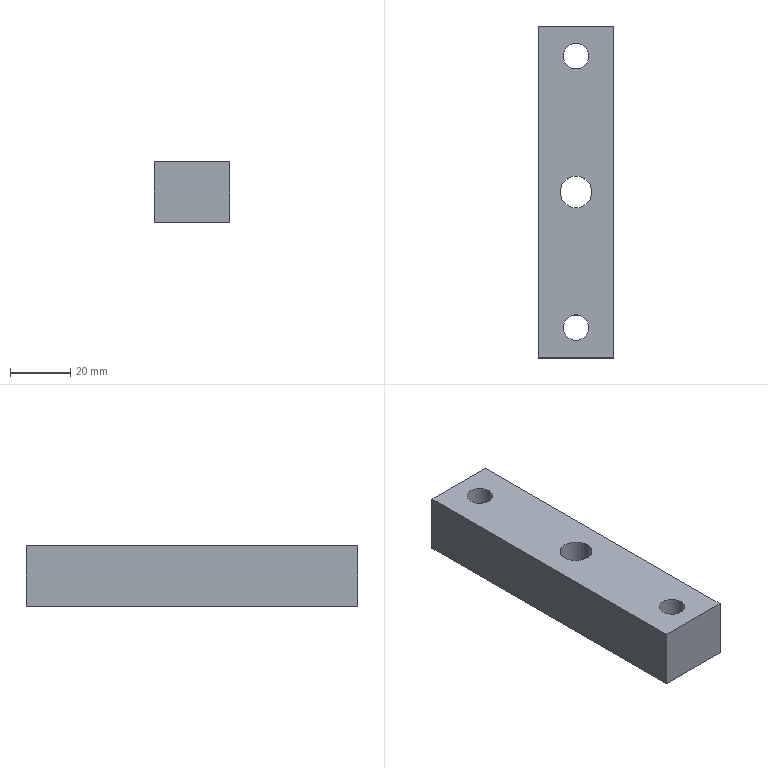Part | SolidWorks | features ICE 2, Extrusion 1, HoleWzd 1 | 1 solid | 18 faces | box 25 x 110 x 20 mm | volume 49479 mm3 | cylinder 10 | plane 8 | commonest cylinder face diameters 8.5 x4 13 x4 10.5 x2
STEP:
#1=CARTESIAN_POINT('',(5.25,0.,20.));
#2=VERTEX_POINT('',#1);
#3=CARTESIAN_POINT('',(-5.25,0.,20.));
#4=VERTEX_POINT('',#3);
#5=CARTESIAN_POINT('',(0.,0.,20.));
#6=DIRECTION('',(0.,0.,-1.));
#7=DIRECTION('',(-1.,0.,0.));
#8=AXIS2_PLACEMENT_3D('',#5,#6,#7);
#9=CIRCLE('',#8,5.25);
#10=EDGE_CURVE('',#2,#4,#9,.T.);
#11=ORIENTED_EDGE('',*,*,#10,.F.);
#12=CARTESIAN_POINT('',(5.25,0.,0.));
#13=VERTEX_POINT('',#12);
#14=CARTESIAN_POINT('',(5.25,0.,0.));
#15=DIRECTION('',(0.,0.,-1.));
#16=VECTOR('',#15,1000.);
#17=LINE('',#14,#16);
#18=EDGE_CURVE('',#2,#13,#17,.T.);
#19=ORIENTED_EDGE('',*,*,#18,.T.);
#20=CARTESIAN_POINT('',(-5.25,0.,0.));
#21=VERTEX_POINT('',#20);
#22=CARTESIAN_POINT('',(0.,0.,0.));
#23=DIRECTION('',(0.,0.,-1.));
#24=DIRECTION('',(-1.,0.,0.));
#25=AXIS2_PLACEMENT_3D('',#22,#23,#24);
#26=CIRCLE('',#25,5.25);
#27=EDGE_CURVE('',#13,#21,#26,.T.);
#28=ORIENTED_EDGE('',*,*,#27,.T.);
#29=CARTESIAN_POINT('',(-5.25,0.,0.));
#30=DIRECTION('',(0.,0.,-1.));
#31=VECTOR('',#30,1000.);
#32=LINE('',#29,#31);
#33=EDGE_CURVE('',#4,#21,#32,.T.);
#34=ORIENTED_EDGE('',*,*,#33,.F.);
#35=EDGE_LOOP('',(#11,#19,#28,#34));
#36=FACE_OUTER_BOUND('',#35,.T.);
#37=CARTESIAN_POINT('',(0.,0.,0.));
#38=DIRECTION('',(0.,0.,-1.));
#39=DIRECTION('',(-1.,0.,0.));
#40=AXIS2_PLACEMENT_3D('',#37,#38,#39);
#41=CYLINDRICAL_SURFACE('',#40,5.25);
#42=ADVANCED_FACE('',(#36),#41,.F.);
#43=CARTESIAN_POINT('',(6.5,-45.,10.));
#44=VERTEX_POINT('',#43);
#45=CARTESIAN_POINT('',(-6.5,-45.,10.));
#46=VERTEX_POINT('',#45);
#47=CARTESIAN_POINT('',(0.,-45.,10.));
#48=DIRECTION('',(0.,0.,-1.));
#49=DIRECTION('',(-1.,0.,0.));
#50=AXIS2_PLACEMENT_3D('',#47,#48,#49);
#51=CIRCLE('',#50,6.5);
#52=EDGE_CURVE('',#44,#46,#51,.T.);
#53=ORIENTED_EDGE('',*,*,#52,.F.);
#54=CARTESIAN_POINT('',(6.5,-45.,0.));
#55=VERTEX_POINT('',#54);
#56=CARTESIAN_POINT('',(6.5,-45.,10.));
#57=DIRECTION('',(0.,0.,-1.));
#58=VECTOR('',#57,1000.);
#59=LINE('',#56,#58);
#60=EDGE_CURVE('',#44,#55,#59,.T.);
#61=ORIENTED_EDGE('',*,*,#60,.T.);
#62=CARTESIAN_POINT('',(-6.5,-45.,0.));
#63=VERTEX_POINT('',#62);
#64=CARTESIAN_POINT('',(0.,-45.,0.));
#65=DIRECTION('',(0.,0.,-1.));
#66=DIRECTION('',(-1.,0.,0.));
#67=AXIS2_PLACEMENT_3D('',#64,#65,#66);
#68=CIRCLE('',#67,6.5);
#69=EDGE_CURVE('',#55,#63,#68,.T.);
#70=ORIENTED_EDGE('',*,*,#69,.T.);
#71=CARTESIAN_POINT('',(-6.5,-45.,10.));
#72=DIRECTION('',(0.,0.,-1.));
#73=VECTOR('',#72,1000.);
#74=LINE('',#71,#73);
#75=EDGE_CURVE('',#46,#63,#74,.T.);
#76=ORIENTED_EDGE('',*,*,#75,.F.);
#77=EDGE_LOOP('',(#53,#61,#70,#76));
#78=FACE_OUTER_BOUND('',#77,.T.);
#79=CARTESIAN_POINT('',(0.,-45.,10.));
#80=DIRECTION('',(0.,0.,-1.));
#81=DIRECTION('',(-1.,0.,0.));
#82=AXIS2_PLACEMENT_3D('',#79,#80,#81);
#83=CYLINDRICAL_SURFACE('',#82,6.5);
#84=ADVANCED_FACE('',(#78),#83,.F.);
#85=CARTESIAN_POINT('',(6.5,45.,10.));
#86=VERTEX_POINT('',#85);
#87=CARTESIAN_POINT('',(-6.5,45.,10.));
#88=VERTEX_POINT('',#87);
#89=CARTESIAN_POINT('',(0.,45.,10.));
#90=DIRECTION('',(0.,0.,-1.));
#91=DIRECTION('',(-1.,0.,0.));
#92=AXIS2_PLACEMENT_3D('',#89,#90,#91);
#93=CIRCLE('',#92,6.5);
#94=EDGE_CURVE('',#86,#88,#93,.T.);
#95=ORIENTED_EDGE('',*,*,#94,.F.);
#96=CARTESIAN_POINT('',(6.5,45.,0.));
#97=VERTEX_POINT('',#96);
#98=CARTESIAN_POINT('',(6.5,45.,10.));
#99=DIRECTION('',(0.,0.,-1.));
#100=VECTOR('',#99,1000.);
#101=LINE('',#98,#100);
#102=EDGE_CURVE('',#86,#97,#101,.T.);
#103=ORIENTED_EDGE('',*,*,#102,.T.);
#104=CARTESIAN_POINT('',(-6.5,45.,0.));
#105=VERTEX_POINT('',#104);
#106=CARTESIAN_POINT('',(0.,45.,0.));
#107=DIRECTION('',(0.,0.,-1.));
#108=DIRECTION('',(-1.,0.,0.));
#109=AXIS2_PLACEMENT_3D('',#106,#107,#108);
#110=CIRCLE('',#109,6.5);
#111=EDGE_CURVE('',#97,#105,#110,.T.);
#112=ORIENTED_EDGE('',*,*,#111,.T.);
#113=CARTESIAN_POINT('',(-6.5,45.,10.));
#114=DIRECTION('',(0.,0.,-1.));
#115=VECTOR('',#114,1000.);
#116=LINE('',#113,#115);
#117=EDGE_CURVE('',#88,#105,#116,.T.);
#118=ORIENTED_EDGE('',*,*,#117,.F.);
#119=EDGE_LOOP('',(#95,#103,#112,#118));
#120=FACE_OUTER_BOUND('',#119,.T.);
#121=CARTESIAN_POINT('',(0.,45.,10.));
#122=DIRECTION('',(0.,0.,-1.));
#123=DIRECTION('',(-1.,0.,0.));
#124=AXIS2_PLACEMENT_3D('',#121,#122,#123);
#125=CYLINDRICAL_SURFACE('',#124,6.5);
#126=ADVANCED_FACE('',(#120),#125,.F.);
#127=CARTESIAN_POINT('',(-4.25,45.,10.));
#128=VERTEX_POINT('',#127);
#129=CARTESIAN_POINT('',(4.25,45.,10.));
#130=VERTEX_POINT('',#129);
#131=CARTESIAN_POINT('',(0.,45.,10.));
#132=DIRECTION('',(0.,0.,1.));
#133=DIRECTION('',(-1.,0.,0.));
#134=AXIS2_PLACEMENT_3D('',#131,#132,#133);
#135=CIRCLE('',#134,4.25);
#136=EDGE_CURVE('',#128,#130,#135,.T.);
#137=ORIENTED_EDGE('',*,*,#136,.F.);
#138=CARTESIAN_POINT('',(-4.25,45.,20.));
#139=VERTEX_POINT('',#138);
#140=CARTESIAN_POINT('',(-4.25,45.,-10.));
#141=DIRECTION('',(0.,0.,1.));
#142=VECTOR('',#141,1000.);
#143=LINE('',#140,#142);
#144=EDGE_CURVE('',#128,#139,#143,.T.);
#145=ORIENTED_EDGE('',*,*,#144,.T.);
#146=CARTESIAN_POINT('',(4.25,45.,20.));
#147=VERTEX_POINT('',#146);
#148=CARTESIAN_POINT('',(0.,45.,20.));
#149=DIRECTION('',(0.,0.,1.));
#150=DIRECTION('',(1.,0.,0.));
#151=AXIS2_PLACEMENT_3D('',#148,#149,#150);
#152=CIRCLE('',#151,4.25);
#153=EDGE_CURVE('',#139,#147,#152,.T.);
#154=ORIENTED_EDGE('',*,*,#153,.T.);
#155=CARTESIAN_POINT('',(4.25,45.,-10.));
#156=DIRECTION('',(0.,0.,1.));
#157=VECTOR('',#156,1000.);
#158=LINE('',#155,#157);
#159=EDGE_CURVE('',#130,#147,#158,.T.);
#160=ORIENTED_EDGE('',*,*,#159,.F.);
#161=EDGE_LOOP('',(#137,#145,#154,#160));
#162=FACE_OUTER_BOUND('',#161,.T.);
#163=CARTESIAN_POINT('',(0.,45.,-10.));
#164=DIRECTION('',(0.,0.,1.));
#165=DIRECTION('',(1.,0.,0.));
#166=AXIS2_PLACEMENT_3D('',#163,#164,#165);
#167=CYLINDRICAL_SURFACE('',#166,4.25);
#168=ADVANCED_FACE('',(#162),#167,.F.);
#169=CARTESIAN_POINT('',(-4.25,-45.,10.));
#170=VERTEX_POINT('',#169);
#171=CARTESIAN_POINT('',(4.25,-45.,10.));
#172=VERTEX_POINT('',#171);
#173=CARTESIAN_POINT('',(0.,-45.,10.));
#174=DIRECTION('',(0.,0.,1.));
#175=DIRECTION('',(-1.,0.,0.));
#176=AXIS2_PLACEMENT_3D('',#173,#174,#175);
#177=CIRCLE('',#176,4.25);
#178=EDGE_CURVE('',#170,#172,#177,.T.);
#179=ORIENTED_EDGE('',*,*,#178,.F.);
#180=CARTESIAN_POINT('',(-4.25,-45.,20.));
#181=VERTEX_POINT('',#180);
#182=CARTESIAN_POINT('',(-4.25,-45.,-10.));
#183=DIRECTION('',(0.,0.,1.));
#184=VECTOR('',#183,1000.);
#185=LINE('',#182,#184);
#186=EDGE_CURVE('',#170,#181,#185,.T.);
#187=ORIENTED_EDGE('',*,*,#186,.T.);
#188=CARTESIAN_POINT('',(4.25,-45.,20.));
#189=VERTEX_POINT('',#188);
#190=CARTESIAN_POINT('',(0.,-45.,20.));
#191=DIRECTION('',(0.,0.,1.));
#192=DIRECTION('',(1.,0.,0.));
#193=AXIS2_PLACEMENT_3D('',#190,#191,#192);
#194=CIRCLE('',#193,4.25);
#195=EDGE_CURVE('',#181,#189,#194,.T.);
#196=ORIENTED_EDGE('',*,*,#195,.T.);
#197=CARTESIAN_POINT('',(4.25,-45.,-10.));
#198=DIRECTION('',(0.,0.,1.));
#199=VECTOR('',#198,1000.);
#200=LINE('',#197,#199);
#201=EDGE_CURVE('',#172,#189,#200,.T.);
#202=ORIENTED_EDGE('',*,*,#201,.F.);
#203=EDGE_LOOP('',(#179,#187,#196,#202));
#204=FACE_OUTER_BOUND('',#203,.T.);
#205=CARTESIAN_POINT('',(0.,-45.,-10.));
#206=DIRECTION('',(0.,0.,1.));
#207=DIRECTION('',(1.,0.,0.));
#208=AXIS2_PLACEMENT_3D('',#205,#206,#207);
#209=CYLINDRICAL_SURFACE('',#208,4.25);
#210=ADVANCED_FACE('',(#204),#209,.F.);
#211=ORIENTED_EDGE('',*,*,#186,.F.);
#212=CARTESIAN_POINT('',(0.,-45.,10.));
#213=DIRECTION('',(0.,0.,1.));
#214=DIRECTION('',(-1.,0.,0.));
#215=AXIS2_PLACEMENT_3D('',#212,#213,#214);
#216=CIRCLE('',#215,4.25);
#217=EDGE_CURVE('',#172,#170,#216,.T.);
#218=ORIENTED_EDGE('',*,*,#217,.F.);
#219=ORIENTED_EDGE('',*,*,#201,.T.);
#220=CARTESIAN_POINT('',(0.,-45.,20.));
#221=DIRECTION('',(0.,0.,1.));
#222=DIRECTION('',(1.,0.,0.));
#223=AXIS2_PLACEMENT_3D('',#220,#221,#222);
#224=CIRCLE('',#223,4.25);
#225=EDGE_CURVE('',#189,#181,#224,.T.);
#226=ORIENTED_EDGE('',*,*,#225,.T.);
#227=EDGE_LOOP('',(#211,#218,#219,#226));
#228=FACE_OUTER_BOUND('',#227,.T.);
#229=CARTESIAN_POINT('',(0.,-45.,-10.));
#230=DIRECTION('',(0.,0.,1.));
#231=DIRECTION('',(1.,0.,0.));
#232=AXIS2_PLACEMENT_3D('',#229,#230,#231);
#233=CYLINDRICAL_SURFACE('',#232,4.25);
#234=ADVANCED_FACE('',(#228),#233,.F.);
#235=ORIENTED_EDGE('',*,*,#144,.F.);
#236=CARTESIAN_POINT('',(0.,45.,10.));
#237=DIRECTION('',(0.,0.,1.));
#238=DIRECTION('',(-1.,0.,0.));
#239=AXIS2_PLACEMENT_3D('',#236,#237,#238);
#240=CIRCLE('',#239,4.25);
#241=EDGE_CURVE('',#130,#128,#240,.T.);
#242=ORIENTED_EDGE('',*,*,#241,.F.);
#243=ORIENTED_EDGE('',*,*,#159,.T.);
#244=CARTESIAN_POINT('',(0.,45.,20.));
#245=DIRECTION('',(0.,0.,1.));
#246=DIRECTION('',(1.,0.,0.));
#247=AXIS2_PLACEMENT_3D('',#244,#245,#246);
#248=CIRCLE('',#247,4.25);
#249=EDGE_CURVE('',#147,#139,#248,.T.);
#250=ORIENTED_EDGE('',*,*,#249,.T.);
#251=EDGE_LOOP('',(#235,#242,#243,#250));
#252=FACE_OUTER_BOUND('',#251,.T.);
#253=CARTESIAN_POINT('',(0.,45.,-10.));
#254=DIRECTION('',(0.,0.,1.));
#255=DIRECTION('',(1.,0.,0.));
#256=AXIS2_PLACEMENT_3D('',#253,#254,#255);
#257=CYLINDRICAL_SURFACE('',#256,4.25);
#258=ADVANCED_FACE('',(#252),#257,.F.);
#259=CARTESIAN_POINT('',(12.5,-55.,0.));
#260=VERTEX_POINT('',#259);
#261=CARTESIAN_POINT('',(12.5,55.,0.));
#262=VERTEX_POINT('',#261);
#263=CARTESIAN_POINT('',(12.5,-55.,0.));
#264=DIRECTION('',(0.,1.,0.));
#265=VECTOR('',#264,1000.);
#266=LINE('',#263,#265);
#267=EDGE_CURVE('',#260,#262,#266,.T.);
#268=ORIENTED_EDGE('',*,*,#267,.T.);
#269=CARTESIAN_POINT('',(12.5,55.,20.));
#270=VERTEX_POINT('',#269);
#271=CARTESIAN_POINT('',(12.5,55.,20.));
#272=DIRECTION('',(0.,0.,-1.));
#273=VECTOR('',#272,1000.);
#274=LINE('',#271,#273);
#275=EDGE_CURVE('',#270,#262,#274,.T.);
#276=ORIENTED_EDGE('',*,*,#275,.F.);
#277=CARTESIAN_POINT('',(12.5,-55.,20.));
#278=VERTEX_POINT('',#277);
#279=CARTESIAN_POINT('',(12.5,-55.,20.));
#280=DIRECTION('',(0.,1.,0.));
#281=VECTOR('',#280,1000.);
#282=LINE('',#279,#281);
#283=EDGE_CURVE('',#278,#270,#282,.T.);
#284=ORIENTED_EDGE('',*,*,#283,.F.);
#285=CARTESIAN_POINT('',(12.5,-55.,20.));
#286=DIRECTION('',(0.,0.,-1.));
#287=VECTOR('',#286,1000.);
#288=LINE('',#285,#287);
#289=EDGE_CURVE('',#278,#260,#288,.T.);
#290=ORIENTED_EDGE('',*,*,#289,.T.);
#291=EDGE_LOOP('',(#268,#276,#284,#290));
#292=FACE_OUTER_BOUND('',#291,.T.);
#293=CARTESIAN_POINT('',(12.5,-55.,20.));
#294=DIRECTION('',(-1.,0.,0.));
#295=DIRECTION('',(0.,0.,1.));
#296=AXIS2_PLACEMENT_3D('',#293,#294,#295);
#297=PLANE('',#296);
#298=ADVANCED_FACE('',(#292),#297,.F.);
#299=CARTESIAN_POINT('',(-12.5,55.,0.));
#300=VERTEX_POINT('',#299);
#301=CARTESIAN_POINT('',(-12.5,55.,0.));
#302=DIRECTION('',(-1.,0.,0.));
#303=VECTOR('',#302,1000.);
#304=LINE('',#301,#303);
#305=EDGE_CURVE('',#262,#300,#304,.T.);
#306=ORIENTED_EDGE('',*,*,#305,.T.);
#307=CARTESIAN_POINT('',(-12.5,55.,20.));
#308=VERTEX_POINT('',#307);
#309=CARTESIAN_POINT('',(-12.5,55.,20.));
#310=DIRECTION('',(0.,0.,-1.));
#311=VECTOR('',#310,1000.);
#312=LINE('',#309,#311);
#313=EDGE_CURVE('',#308,#300,#312,.T.);
#314=ORIENTED_EDGE('',*,*,#313,.F.);
#315=CARTESIAN_POINT('',(-12.5,55.,20.));
#316=DIRECTION('',(-1.,0.,0.));
#317=VECTOR('',#316,1000.);
#318=LINE('',#315,#317);
#319=EDGE_CURVE('',#270,#308,#318,.T.);
#320=ORIENTED_EDGE('',*,*,#319,.F.);
#321=ORIENTED_EDGE('',*,*,#275,.T.);
#322=EDGE_LOOP('',(#306,#314,#320,#321));
#323=FACE_OUTER_BOUND('',#322,.T.);
#324=CARTESIAN_POINT('',(-12.5,55.,20.));
#325=DIRECTION('',(0.,-1.,0.));
#326=DIRECTION('',(0.,0.,-1.));
#327=AXIS2_PLACEMENT_3D('',#324,#325,#326);
#328=PLANE('',#327);
#329=ADVANCED_FACE('',(#323),#328,.F.);
#330=CARTESIAN_POINT('',(-12.5,-55.,0.));
#331=VERTEX_POINT('',#330);
#332=CARTESIAN_POINT('',(-12.5,-55.,0.));
#333=DIRECTION('',(0.,-1.,0.));
#334=VECTOR('',#333,1000.);
#335=LINE('',#332,#334);
#336=EDGE_CURVE('',#300,#331,#335,.T.);
#337=ORIENTED_EDGE('',*,*,#336,.T.);
#338=CARTESIAN_POINT('',(-12.5,-55.,20.));
#339=VERTEX_POINT('',#338);
#340=CARTESIAN_POINT('',(-12.5,-55.,20.));
#341=DIRECTION('',(0.,0.,-1.));
#342=VECTOR('',#341,1000.);
#343=LINE('',#340,#342);
#344=EDGE_CURVE('',#339,#331,#343,.T.);
#345=ORIENTED_EDGE('',*,*,#344,.F.);
#346=CARTESIAN_POINT('',(-12.5,-55.,20.));
#347=DIRECTION('',(0.,-1.,0.));
#348=VECTOR('',#347,1000.);
#349=LINE('',#346,#348);
#350=EDGE_CURVE('',#308,#339,#349,.T.);
#351=ORIENTED_EDGE('',*,*,#350,.F.);
#352=ORIENTED_EDGE('',*,*,#313,.T.);
#353=EDGE_LOOP('',(#337,#345,#351,#352));
#354=FACE_OUTER_BOUND('',#353,.T.);
#355=CARTESIAN_POINT('',(-12.5,-55.,20.));
#356=DIRECTION('',(1.,0.,0.));
#357=DIRECTION('',(0.,0.,-1.));
#358=AXIS2_PLACEMENT_3D('',#355,#356,#357);
#359=PLANE('',#358);
#360=ADVANCED_FACE('',(#354),#359,.F.);
#361=CARTESIAN_POINT('',(-12.5,-55.,0.));
#362=DIRECTION('',(1.,0.,0.));
#363=VECTOR('',#362,1000.);
#364=LINE('',#361,#363);
#365=EDGE_CURVE('',#331,#260,#364,.T.);
#366=ORIENTED_EDGE('',*,*,#365,.T.);
#367=ORIENTED_EDGE('',*,*,#289,.F.);
#368=CARTESIAN_POINT('',(-12.5,-55.,20.));
#369=DIRECTION('',(1.,0.,0.));
#370=VECTOR('',#369,1000.);
#371=LINE('',#368,#370);
#372=EDGE_CURVE('',#339,#278,#371,.T.);
#373=ORIENTED_EDGE('',*,*,#372,.F.);
#374=ORIENTED_EDGE('',*,*,#344,.T.);
#375=EDGE_LOOP('',(#366,#367,#373,#374));
#376=FACE_OUTER_BOUND('',#375,.T.);
#377=CARTESIAN_POINT('',(-12.5,-55.,20.));
#378=DIRECTION('',(0.,1.,0.));
#379=DIRECTION('',(0.,0.,1.));
#380=AXIS2_PLACEMENT_3D('',#377,#378,#379);
#381=PLANE('',#380);
#382=ADVANCED_FACE('',(#376),#381,.F.);
#383=CARTESIAN_POINT('',(0.,0.,20.));
#384=DIRECTION('',(0.,0.,-1.));
#385=DIRECTION('',(-1.,0.,0.));
#386=AXIS2_PLACEMENT_3D('',#383,#384,#385);
#387=CIRCLE('',#386,5.25);
#388=EDGE_CURVE('',#4,#2,#387,.T.);
#389=ORIENTED_EDGE('',*,*,#388,.T.);
#390=ORIENTED_EDGE('',*,*,#10,.T.);
#391=EDGE_LOOP('',(#389,#390));
#392=FACE_BOUND('',#391,.T.);
#393=ORIENTED_EDGE('',*,*,#225,.F.);
#394=ORIENTED_EDGE('',*,*,#195,.F.);
#395=EDGE_LOOP('',(#393,#394));
#396=FACE_BOUND('',#395,.T.);
#397=ORIENTED_EDGE('',*,*,#249,.F.);
#398=ORIENTED_EDGE('',*,*,#153,.F.);
#399=EDGE_LOOP('',(#397,#398));
#400=FACE_BOUND('',#399,.T.);
#401=ORIENTED_EDGE('',*,*,#283,.T.);
#402=ORIENTED_EDGE('',*,*,#319,.T.);
#403=ORIENTED_EDGE('',*,*,#350,.T.);
#404=ORIENTED_EDGE('',*,*,#372,.T.);
#405=EDGE_LOOP('',(#401,#402,#403,#404));
#406=FACE_OUTER_BOUND('',#405,.T.);
#407=CARTESIAN_POINT('',(0.,0.,20.));
#408=DIRECTION('',(0.,0.,-1.));
#409=DIRECTION('',(-1.,0.,0.));
#410=AXIS2_PLACEMENT_3D('',#407,#408,#409);
#411=PLANE('',#410);
#412=ADVANCED_FACE('',(#392,#396,#400,#406),#411,.F.);
#413=CARTESIAN_POINT('',(0.,0.,0.));
#414=DIRECTION('',(0.,0.,-1.));
#415=DIRECTION('',(-1.,0.,0.));
#416=AXIS2_PLACEMENT_3D('',#413,#414,#415);
#417=CIRCLE('',#416,5.25);
#418=EDGE_CURVE('',#21,#13,#417,.T.);
#419=ORIENTED_EDGE('',*,*,#418,.F.);
#420=ORIENTED_EDGE('',*,*,#27,.F.);
#421=EDGE_LOOP('',(#419,#420));
#422=FACE_BOUND('',#421,.T.);
#423=CARTESIAN_POINT('',(0.,-45.,0.));
#424=DIRECTION('',(0.,0.,-1.));
#425=DIRECTION('',(-1.,0.,0.));
#426=AXIS2_PLACEMENT_3D('',#423,#424,#425);
#427=CIRCLE('',#426,6.5);
#428=EDGE_CURVE('',#63,#55,#427,.T.);
#429=ORIENTED_EDGE('',*,*,#428,.F.);
#430=ORIENTED_EDGE('',*,*,#69,.F.);
#431=EDGE_LOOP('',(#429,#430));
#432=FACE_BOUND('',#431,.T.);
#433=CARTESIAN_POINT('',(0.,45.,0.));
#434=DIRECTION('',(0.,0.,-1.));
#435=DIRECTION('',(-1.,0.,0.));
#436=AXIS2_PLACEMENT_3D('',#433,#434,#435);
#437=CIRCLE('',#436,6.5);
#438=EDGE_CURVE('',#105,#97,#437,.T.);
#439=ORIENTED_EDGE('',*,*,#438,.F.);
#440=ORIENTED_EDGE('',*,*,#111,.F.);
#441=EDGE_LOOP('',(#439,#440));
#442=FACE_BOUND('',#441,.T.);
#443=ORIENTED_EDGE('',*,*,#267,.F.);
#444=ORIENTED_EDGE('',*,*,#365,.F.);
#445=ORIENTED_EDGE('',*,*,#336,.F.);
#446=ORIENTED_EDGE('',*,*,#305,.F.);
#447=EDGE_LOOP('',(#443,#444,#445,#446));
#448=FACE_OUTER_BOUND('',#447,.T.);
#449=CARTESIAN_POINT('',(0.,0.,0.));
#450=DIRECTION('',(0.,0.,-1.));
#451=DIRECTION('',(-1.,0.,0.));
#452=AXIS2_PLACEMENT_3D('',#449,#450,#451);
#453=PLANE('',#452);
#454=ADVANCED_FACE('',(#422,#432,#442,#448),#453,.T.);
#455=CARTESIAN_POINT('',(0.,45.,10.));
#456=DIRECTION('',(0.,0.,-1.));
#457=DIRECTION('',(-1.,0.,0.));
#458=AXIS2_PLACEMENT_3D('',#455,#456,#457);
#459=CIRCLE('',#458,6.5);
#460=EDGE_CURVE('',#88,#86,#459,.T.);
#461=ORIENTED_EDGE('',*,*,#460,.T.);
#462=ORIENTED_EDGE('',*,*,#94,.T.);
#463=EDGE_LOOP('',(#461,#462));
#464=FACE_OUTER_BOUND('',#463,.T.);
#465=ORIENTED_EDGE('',*,*,#241,.T.);
#466=ORIENTED_EDGE('',*,*,#136,.T.);
#467=EDGE_LOOP('',(#465,#466));
#468=FACE_BOUND('',#467,.T.);
#469=CARTESIAN_POINT('',(0.,45.,10.));
#470=DIRECTION('',(0.,0.,-1.));
#471=DIRECTION('',(-1.,0.,0.));
#472=AXIS2_PLACEMENT_3D('',#469,#470,#471);
#473=PLANE('',#472);
#474=ADVANCED_FACE('',(#464,#468),#473,.T.);
#475=ORIENTED_EDGE('',*,*,#102,.F.);
#476=ORIENTED_EDGE('',*,*,#460,.F.);
#477=ORIENTED_EDGE('',*,*,#117,.T.);
#478=ORIENTED_EDGE('',*,*,#438,.T.);
#479=EDGE_LOOP('',(#475,#476,#477,#478));
#480=FACE_OUTER_BOUND('',#479,.T.);
#481=CARTESIAN_POINT('',(0.,45.,10.));
#482=DIRECTION('',(0.,0.,-1.));
#483=DIRECTION('',(-1.,0.,0.));
#484=AXIS2_PLACEMENT_3D('',#481,#482,#483);
#485=CYLINDRICAL_SURFACE('',#484,6.5);
#486=ADVANCED_FACE('',(#480),#485,.F.);
#487=CARTESIAN_POINT('',(0.,-45.,10.));
#488=DIRECTION('',(0.,0.,-1.));
#489=DIRECTION('',(-1.,0.,0.));
#490=AXIS2_PLACEMENT_3D('',#487,#488,#489);
#491=CIRCLE('',#490,6.5);
#492=EDGE_CURVE('',#46,#44,#491,.T.);
#493=ORIENTED_EDGE('',*,*,#492,.T.);
#494=ORIENTED_EDGE('',*,*,#52,.T.);
#495=EDGE_LOOP('',(#493,#494));
#496=FACE_OUTER_BOUND('',#495,.T.);
#497=ORIENTED_EDGE('',*,*,#217,.T.);
#498=ORIENTED_EDGE('',*,*,#178,.T.);
#499=EDGE_LOOP('',(#497,#498));
#500=FACE_BOUND('',#499,.T.);
#501=CARTESIAN_POINT('',(0.,-45.,10.));
#502=DIRECTION('',(0.,0.,-1.));
#503=DIRECTION('',(-1.,0.,0.));
#504=AXIS2_PLACEMENT_3D('',#501,#502,#503);
#505=PLANE('',#504);
#506=ADVANCED_FACE('',(#496,#500),#505,.T.);
#507=ORIENTED_EDGE('',*,*,#60,.F.);
#508=ORIENTED_EDGE('',*,*,#492,.F.);
#509=ORIENTED_EDGE('',*,*,#75,.T.);
#510=ORIENTED_EDGE('',*,*,#428,.T.);
#511=EDGE_LOOP('',(#507,#508,#509,#510));
#512=FACE_OUTER_BOUND('',#511,.T.);
#513=CARTESIAN_POINT('',(0.,-45.,10.));
#514=DIRECTION('',(0.,0.,-1.));
#515=DIRECTION('',(-1.,0.,0.));
#516=AXIS2_PLACEMENT_3D('',#513,#514,#515);
#517=CYLINDRICAL_SURFACE('',#516,6.5);
#518=ADVANCED_FACE('',(#512),#517,.F.);
#519=ORIENTED_EDGE('',*,*,#18,.F.);
#520=ORIENTED_EDGE('',*,*,#388,.F.);
#521=ORIENTED_EDGE('',*,*,#33,.T.);
#522=ORIENTED_EDGE('',*,*,#418,.T.);
#523=EDGE_LOOP('',(#519,#520,#521,#522));
#524=FACE_OUTER_BOUND('',#523,.T.);
#525=CARTESIAN_POINT('',(0.,0.,0.));
#526=DIRECTION('',(0.,0.,-1.));
#527=DIRECTION('',(-1.,0.,0.));
#528=AXIS2_PLACEMENT_3D('',#525,#526,#527);
#529=CYLINDRICAL_SURFACE('',#528,5.25);
#530=ADVANCED_FACE('',(#524),#529,.F.);
#531=CLOSED_SHELL('',(#42,#84,#126,#168,#210,#234,#258,#298,#329,#360,#382,#412,#454,#474,#486,#506,#518,#530));
#532=MANIFOLD_SOLID_BREP('',#531);
#533=CARTESIAN_POINT('',(0.,0.,0.));
#534=DIRECTION('',(0.,0.,1.));
#535=DIRECTION('',(1.,0.,0.));
#536=AXIS2_PLACEMENT_3D('',#533,#534,#535);
#537=(LENGTH_UNIT()NAMED_UNIT(*)SI_UNIT(.MILLI.,.METRE.));
#538=UNCERTAINTY_MEASURE_WITH_UNIT(LENGTH_MEASURE(0.00001),#537,'','');
#539=(NAMED_UNIT(*)PLANE_ANGLE_UNIT()SI_UNIT($,.RADIAN.));
#540=(NAMED_UNIT(*)SI_UNIT($,.STERADIAN.)SOLID_ANGLE_UNIT());
#541=(GEOMETRIC_REPRESENTATION_CONTEXT(3)GLOBAL_UNCERTAINTY_ASSIGNED_CONTEXT((#538))GLOBAL_UNIT_ASSIGNED_CONTEXT((#537,#539,#540))REPRESENTATION_CONTEXT('',''));
#542=ADVANCED_BREP_SHAPE_REPRESENTATION('',(#532,#536),#541);